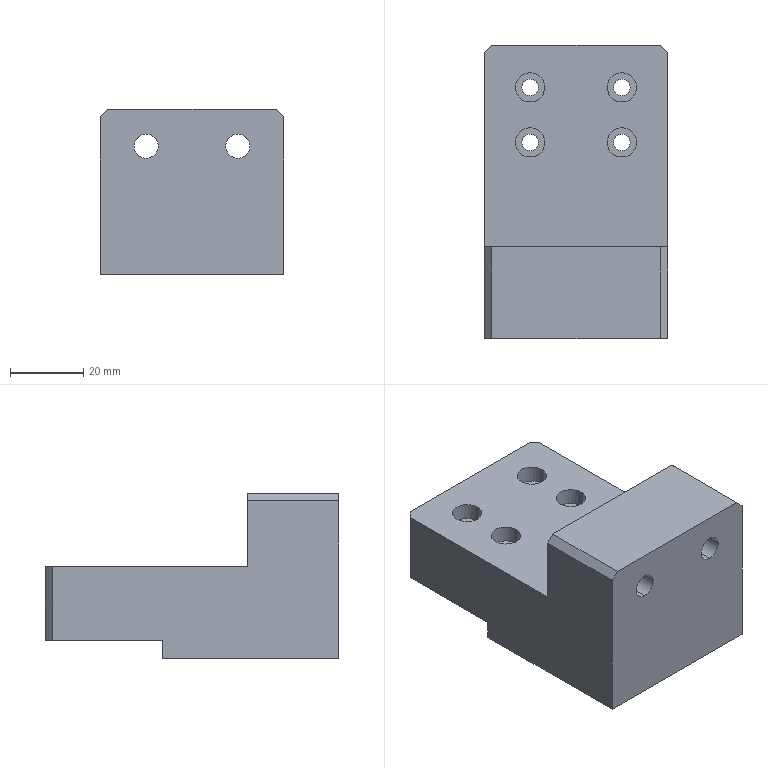Part | STEP file | FBDS-CS-011 | 1 solid | 44 faces | box 50 x 80 x 45 mm | volume 112378 mm3 | cylinder 24 | plane 20 | commonest cylinder face diameters 4.5 x8 8 x8 6.6 x4 11 x4
STEP:
#1=CARTESIAN_POINT('',(-12.5,-21.8,14.5));
#2=VERTEX_POINT('',#1);
#3=CARTESIAN_POINT('',(-12.5,-21.8,25.5));
#4=VERTEX_POINT('',#3);
#5=CARTESIAN_POINT('',(-12.5,-21.8,20.));
#6=DIRECTION('',(0.,1.,0.));
#7=DIRECTION('',(0.,0.,1.));
#8=AXIS2_PLACEMENT_3D('',#5,#6,#7);
#9=CIRCLE('',#8,5.5);
#10=EDGE_CURVE('',#2,#4,#9,.T.);
#11=ORIENTED_EDGE('',*,*,#10,.F.);
#12=CARTESIAN_POINT('',(-12.5,-15.,14.5));
#13=VERTEX_POINT('',#12);
#14=CARTESIAN_POINT('',(-12.5,-15.,14.5));
#15=DIRECTION('',(0.,1.,0.));
#16=VECTOR('',#15,1000.);
#17=LINE('',#14,#16);
#18=EDGE_CURVE('',#2,#13,#17,.T.);
#19=ORIENTED_EDGE('',*,*,#18,.T.);
#20=CARTESIAN_POINT('',(-12.5,-15.,25.5));
#21=VERTEX_POINT('',#20);
#22=CARTESIAN_POINT('',(-12.5,-15.,20.));
#23=DIRECTION('',(0.,1.,0.));
#24=DIRECTION('',(0.,0.,1.));
#25=AXIS2_PLACEMENT_3D('',#22,#23,#24);
#26=CIRCLE('',#25,5.5);
#27=EDGE_CURVE('',#13,#21,#26,.T.);
#28=ORIENTED_EDGE('',*,*,#27,.T.);
#29=CARTESIAN_POINT('',(-12.5,-15.,25.5));
#30=DIRECTION('',(0.,1.,0.));
#31=VECTOR('',#30,1000.);
#32=LINE('',#29,#31);
#33=EDGE_CURVE('',#4,#21,#32,.T.);
#34=ORIENTED_EDGE('',*,*,#33,.F.);
#35=EDGE_LOOP('',(#11,#19,#28,#34));
#36=FACE_OUTER_BOUND('',#35,.T.);
#37=CARTESIAN_POINT('',(-12.5,-15.,20.));
#38=DIRECTION('',(0.,1.,0.));
#39=DIRECTION('',(0.,0.,1.));
#40=AXIS2_PLACEMENT_3D('',#37,#38,#39);
#41=CYLINDRICAL_SURFACE('',#40,5.5);
#42=ADVANCED_FACE('',(#36),#41,.F.);
#43=CARTESIAN_POINT('',(-12.5,-40.,16.7));
#44=VERTEX_POINT('',#43);
#45=CARTESIAN_POINT('',(-12.5,-40.,23.3));
#46=VERTEX_POINT('',#45);
#47=CARTESIAN_POINT('',(-12.5,-40.,20.));
#48=DIRECTION('',(0.,1.,0.));
#49=DIRECTION('',(0.,0.,1.));
#50=AXIS2_PLACEMENT_3D('',#47,#48,#49);
#51=CIRCLE('',#50,3.3);
#52=EDGE_CURVE('',#44,#46,#51,.T.);
#53=ORIENTED_EDGE('',*,*,#52,.F.);
#54=CARTESIAN_POINT('',(-12.5,-21.8,16.7));
#55=VERTEX_POINT('',#54);
#56=CARTESIAN_POINT('',(-12.5,-15.,16.7));
#57=DIRECTION('',(0.,1.,0.));
#58=VECTOR('',#57,1000.);
#59=LINE('',#56,#58);
#60=EDGE_CURVE('',#44,#55,#59,.T.);
#61=ORIENTED_EDGE('',*,*,#60,.T.);
#62=CARTESIAN_POINT('',(-12.5,-21.8,23.3));
#63=VERTEX_POINT('',#62);
#64=CARTESIAN_POINT('',(-12.5,-21.8,20.));
#65=DIRECTION('',(0.,1.,0.));
#66=DIRECTION('',(0.,0.,1.));
#67=AXIS2_PLACEMENT_3D('',#64,#65,#66);
#68=CIRCLE('',#67,3.3);
#69=EDGE_CURVE('',#55,#63,#68,.T.);
#70=ORIENTED_EDGE('',*,*,#69,.T.);
#71=CARTESIAN_POINT('',(-12.5,-15.,23.3));
#72=DIRECTION('',(0.,1.,0.));
#73=VECTOR('',#72,1000.);
#74=LINE('',#71,#73);
#75=EDGE_CURVE('',#46,#63,#74,.T.);
#76=ORIENTED_EDGE('',*,*,#75,.F.);
#77=EDGE_LOOP('',(#53,#61,#70,#76));
#78=FACE_OUTER_BOUND('',#77,.T.);
#79=CARTESIAN_POINT('',(-12.5,-15.,20.));
#80=DIRECTION('',(0.,1.,0.));
#81=DIRECTION('',(0.,0.,1.));
#82=AXIS2_PLACEMENT_3D('',#79,#80,#81);
#83=CYLINDRICAL_SURFACE('',#82,3.3);
#84=ADVANCED_FACE('',(#78),#83,.F.);
#85=CARTESIAN_POINT('',(12.5,-21.8,14.5));
#86=VERTEX_POINT('',#85);
#87=CARTESIAN_POINT('',(12.5,-21.8,25.5));
#88=VERTEX_POINT('',#87);
#89=CARTESIAN_POINT('',(12.5,-21.8,20.));
#90=DIRECTION('',(0.,1.,0.));
#91=DIRECTION('',(0.,0.,1.));
#92=AXIS2_PLACEMENT_3D('',#89,#90,#91);
#93=CIRCLE('',#92,5.5);
#94=EDGE_CURVE('',#86,#88,#93,.T.);
#95=ORIENTED_EDGE('',*,*,#94,.F.);
#96=CARTESIAN_POINT('',(12.5,-15.,14.5));
#97=VERTEX_POINT('',#96);
#98=CARTESIAN_POINT('',(12.5,-15.,14.5));
#99=DIRECTION('',(0.,1.,0.));
#100=VECTOR('',#99,1000.);
#101=LINE('',#98,#100);
#102=EDGE_CURVE('',#86,#97,#101,.T.);
#103=ORIENTED_EDGE('',*,*,#102,.T.);
#104=CARTESIAN_POINT('',(12.5,-15.,25.5));
#105=VERTEX_POINT('',#104);
#106=CARTESIAN_POINT('',(12.5,-15.,20.));
#107=DIRECTION('',(0.,1.,0.));
#108=DIRECTION('',(0.,0.,1.));
#109=AXIS2_PLACEMENT_3D('',#106,#107,#108);
#110=CIRCLE('',#109,5.5);
#111=EDGE_CURVE('',#97,#105,#110,.T.);
#112=ORIENTED_EDGE('',*,*,#111,.T.);
#113=CARTESIAN_POINT('',(12.5,-15.,25.5));
#114=DIRECTION('',(0.,1.,0.));
#115=VECTOR('',#114,1000.);
#116=LINE('',#113,#115);
#117=EDGE_CURVE('',#88,#105,#116,.T.);
#118=ORIENTED_EDGE('',*,*,#117,.F.);
#119=EDGE_LOOP('',(#95,#103,#112,#118));
#120=FACE_OUTER_BOUND('',#119,.T.);
#121=CARTESIAN_POINT('',(12.5,-15.,20.));
#122=DIRECTION('',(0.,1.,0.));
#123=DIRECTION('',(0.,0.,1.));
#124=AXIS2_PLACEMENT_3D('',#121,#122,#123);
#125=CYLINDRICAL_SURFACE('',#124,5.5);
#126=ADVANCED_FACE('',(#120),#125,.F.);
#127=CARTESIAN_POINT('',(12.5,-40.,16.7));
#128=VERTEX_POINT('',#127);
#129=CARTESIAN_POINT('',(12.5,-40.,23.3));
#130=VERTEX_POINT('',#129);
#131=CARTESIAN_POINT('',(12.5,-40.,20.));
#132=DIRECTION('',(0.,1.,0.));
#133=DIRECTION('',(0.,0.,1.));
#134=AXIS2_PLACEMENT_3D('',#131,#132,#133);
#135=CIRCLE('',#134,3.3);
#136=EDGE_CURVE('',#128,#130,#135,.T.);
#137=ORIENTED_EDGE('',*,*,#136,.F.);
#138=CARTESIAN_POINT('',(12.5,-21.8,16.7));
#139=VERTEX_POINT('',#138);
#140=CARTESIAN_POINT('',(12.5,-15.,16.7));
#141=DIRECTION('',(0.,1.,0.));
#142=VECTOR('',#141,1000.);
#143=LINE('',#140,#142);
#144=EDGE_CURVE('',#128,#139,#143,.T.);
#145=ORIENTED_EDGE('',*,*,#144,.T.);
#146=CARTESIAN_POINT('',(12.5,-21.8,23.3));
#147=VERTEX_POINT('',#146);
#148=CARTESIAN_POINT('',(12.5,-21.8,20.));
#149=DIRECTION('',(0.,1.,0.));
#150=DIRECTION('',(0.,0.,1.));
#151=AXIS2_PLACEMENT_3D('',#148,#149,#150);
#152=CIRCLE('',#151,3.3);
#153=EDGE_CURVE('',#139,#147,#152,.T.);
#154=ORIENTED_EDGE('',*,*,#153,.T.);
#155=CARTESIAN_POINT('',(12.5,-15.,23.3));
#156=DIRECTION('',(0.,1.,0.));
#157=VECTOR('',#156,1000.);
#158=LINE('',#155,#157);
#159=EDGE_CURVE('',#130,#147,#158,.T.);
#160=ORIENTED_EDGE('',*,*,#159,.F.);
#161=EDGE_LOOP('',(#137,#145,#154,#160));
#162=FACE_OUTER_BOUND('',#161,.T.);
#163=CARTESIAN_POINT('',(12.5,-15.,20.));
#164=DIRECTION('',(0.,1.,0.));
#165=DIRECTION('',(0.,0.,1.));
#166=AXIS2_PLACEMENT_3D('',#163,#164,#165);
#167=CYLINDRICAL_SURFACE('',#166,3.3);
#168=ADVANCED_FACE('',(#162),#167,.F.);
#169=CARTESIAN_POINT('',(-16.5,28.5,5.4));
#170=VERTEX_POINT('',#169);
#171=CARTESIAN_POINT('',(-8.5,28.5,5.4));
#172=VERTEX_POINT('',#171);
#173=CARTESIAN_POINT('',(-12.5,28.5,5.4));
#174=DIRECTION('',(0.,0.,1.));
#175=DIRECTION('',(1.,0.,0.));
#176=AXIS2_PLACEMENT_3D('',#173,#174,#175);
#177=CIRCLE('',#176,4.);
#178=EDGE_CURVE('',#170,#172,#177,.T.);
#179=ORIENTED_EDGE('',*,*,#178,.F.);
#180=CARTESIAN_POINT('',(-16.5,28.5,10.));
#181=VERTEX_POINT('',#180);
#182=CARTESIAN_POINT('',(-16.5,28.5,10.));
#183=DIRECTION('',(0.,0.,1.));
#184=VECTOR('',#183,1000.);
#185=LINE('',#182,#184);
#186=EDGE_CURVE('',#170,#181,#185,.T.);
#187=ORIENTED_EDGE('',*,*,#186,.T.);
#188=CARTESIAN_POINT('',(-8.5,28.5,10.));
#189=VERTEX_POINT('',#188);
#190=CARTESIAN_POINT('',(-12.5,28.5,10.));
#191=DIRECTION('',(0.,0.,1.));
#192=DIRECTION('',(1.,0.,0.));
#193=AXIS2_PLACEMENT_3D('',#190,#191,#192);
#194=CIRCLE('',#193,4.);
#195=EDGE_CURVE('',#181,#189,#194,.T.);
#196=ORIENTED_EDGE('',*,*,#195,.T.);
#197=CARTESIAN_POINT('',(-8.5,28.5,10.));
#198=DIRECTION('',(0.,0.,1.));
#199=VECTOR('',#198,1000.);
#200=LINE('',#197,#199);
#201=EDGE_CURVE('',#172,#189,#200,.T.);
#202=ORIENTED_EDGE('',*,*,#201,.F.);
#203=EDGE_LOOP('',(#179,#187,#196,#202));
#204=FACE_OUTER_BOUND('',#203,.T.);
#205=CARTESIAN_POINT('',(-12.5,28.5,10.));
#206=DIRECTION('',(0.,0.,1.));
#207=DIRECTION('',(1.,0.,0.));
#208=AXIS2_PLACEMENT_3D('',#205,#206,#207);
#209=CYLINDRICAL_SURFACE('',#208,4.);
#210=ADVANCED_FACE('',(#204),#209,.F.);
#211=CARTESIAN_POINT('',(-14.75,28.5,-10.));
#212=VERTEX_POINT('',#211);
#213=CARTESIAN_POINT('',(-10.25,28.5,-10.));
#214=VERTEX_POINT('',#213);
#215=CARTESIAN_POINT('',(-12.5,28.5,-10.));
#216=DIRECTION('',(0.,0.,1.));
#217=DIRECTION('',(1.,0.,0.));
#218=AXIS2_PLACEMENT_3D('',#215,#216,#217);
#219=CIRCLE('',#218,2.25);
#220=EDGE_CURVE('',#212,#214,#219,.T.);
#221=ORIENTED_EDGE('',*,*,#220,.F.);
#222=CARTESIAN_POINT('',(-14.75,28.5,5.4));
#223=VERTEX_POINT('',#222);
#224=CARTESIAN_POINT('',(-14.75,28.5,10.));
#225=DIRECTION('',(0.,0.,1.));
#226=VECTOR('',#225,1000.);
#227=LINE('',#224,#226);
#228=EDGE_CURVE('',#212,#223,#227,.T.);
#229=ORIENTED_EDGE('',*,*,#228,.T.);
#230=CARTESIAN_POINT('',(-10.25,28.5,5.4));
#231=VERTEX_POINT('',#230);
#232=CARTESIAN_POINT('',(-12.5,28.5,5.4));
#233=DIRECTION('',(0.,0.,1.));
#234=DIRECTION('',(1.,0.,0.));
#235=AXIS2_PLACEMENT_3D('',#232,#233,#234);
#236=CIRCLE('',#235,2.25);
#237=EDGE_CURVE('',#223,#231,#236,.T.);
#238=ORIENTED_EDGE('',*,*,#237,.T.);
#239=CARTESIAN_POINT('',(-10.25,28.5,10.));
#240=DIRECTION('',(0.,0.,1.));
#241=VECTOR('',#240,1000.);
#242=LINE('',#239,#241);
#243=EDGE_CURVE('',#214,#231,#242,.T.);
#244=ORIENTED_EDGE('',*,*,#243,.F.);
#245=EDGE_LOOP('',(#221,#229,#238,#244));
#246=FACE_OUTER_BOUND('',#245,.T.);
#247=CARTESIAN_POINT('',(-12.5,28.5,10.));
#248=DIRECTION('',(0.,0.,1.));
#249=DIRECTION('',(1.,0.,0.));
#250=AXIS2_PLACEMENT_3D('',#247,#248,#249);
#251=CYLINDRICAL_SURFACE('',#250,2.25);
#252=ADVANCED_FACE('',(#246),#251,.F.);
#253=CARTESIAN_POINT('',(8.5,28.5,5.4));
#254=VERTEX_POINT('',#253);
#255=CARTESIAN_POINT('',(16.5,28.5,5.4));
#256=VERTEX_POINT('',#255);
#257=CARTESIAN_POINT('',(12.5,28.5,5.4));
#258=DIRECTION('',(0.,0.,1.));
#259=DIRECTION('',(1.,0.,0.));
#260=AXIS2_PLACEMENT_3D('',#257,#258,#259);
#261=CIRCLE('',#260,4.);
#262=EDGE_CURVE('',#254,#256,#261,.T.);
#263=ORIENTED_EDGE('',*,*,#262,.F.);
#264=CARTESIAN_POINT('',(8.5,28.5,10.));
#265=VERTEX_POINT('',#264);
#266=CARTESIAN_POINT('',(8.5,28.5,10.));
#267=DIRECTION('',(0.,0.,1.));
#268=VECTOR('',#267,1000.);
#269=LINE('',#266,#268);
#270=EDGE_CURVE('',#254,#265,#269,.T.);
#271=ORIENTED_EDGE('',*,*,#270,.T.);
#272=CARTESIAN_POINT('',(16.5,28.5,10.));
#273=VERTEX_POINT('',#272);
#274=CARTESIAN_POINT('',(12.5,28.5,10.));
#275=DIRECTION('',(0.,0.,1.));
#276=DIRECTION('',(1.,0.,0.));
#277=AXIS2_PLACEMENT_3D('',#274,#275,#276);
#278=CIRCLE('',#277,4.);
#279=EDGE_CURVE('',#265,#273,#278,.T.);
#280=ORIENTED_EDGE('',*,*,#279,.T.);
#281=CARTESIAN_POINT('',(16.5,28.5,10.));
#282=DIRECTION('',(0.,0.,1.));
#283=VECTOR('',#282,1000.);
#284=LINE('',#281,#283);
#285=EDGE_CURVE('',#256,#273,#284,.T.);
#286=ORIENTED_EDGE('',*,*,#285,.F.);
#287=EDGE_LOOP('',(#263,#271,#280,#286));
#288=FACE_OUTER_BOUND('',#287,.T.);
#289=CARTESIAN_POINT('',(12.5,28.5,10.));
#290=DIRECTION('',(0.,0.,1.));
#291=DIRECTION('',(1.,0.,0.));
#292=AXIS2_PLACEMENT_3D('',#289,#290,#291);
#293=CYLINDRICAL_SURFACE('',#292,4.);
#294=ADVANCED_FACE('',(#288),#293,.F.);
#295=CARTESIAN_POINT('',(10.25,28.5,-10.));
#296=VERTEX_POINT('',#295);
#297=CARTESIAN_POINT('',(14.75,28.5,-10.));
#298=VERTEX_POINT('',#297);
#299=CARTESIAN_POINT('',(12.5,28.5,-10.));
#300=DIRECTION('',(0.,0.,1.));
#301=DIRECTION('',(1.,0.,0.));
#302=AXIS2_PLACEMENT_3D('',#299,#300,#301);
#303=CIRCLE('',#302,2.25);
#304=EDGE_CURVE('',#296,#298,#303,.T.);
#305=ORIENTED_EDGE('',*,*,#304,.F.);
#306=CARTESIAN_POINT('',(10.25,28.5,5.4));
#307=VERTEX_POINT('',#306);
#308=CARTESIAN_POINT('',(10.25,28.5,10.));
#309=DIRECTION('',(0.,0.,1.));
#310=VECTOR('',#309,1000.);
#311=LINE('',#308,#310);
#312=EDGE_CURVE('',#296,#307,#311,.T.);
#313=ORIENTED_EDGE('',*,*,#312,.T.);
#314=CARTESIAN_POINT('',(14.75,28.5,5.4));
#315=VERTEX_POINT('',#314);
#316=CARTESIAN_POINT('',(12.5,28.5,5.4));
#317=DIRECTION('',(0.,0.,1.));
#318=DIRECTION('',(1.,0.,0.));
#319=AXIS2_PLACEMENT_3D('',#316,#317,#318);
#320=CIRCLE('',#319,2.25);
#321=EDGE_CURVE('',#307,#315,#320,.T.);
#322=ORIENTED_EDGE('',*,*,#321,.T.);
#323=CARTESIAN_POINT('',(14.75,28.5,10.));
#324=DIRECTION('',(0.,0.,1.));
#325=VECTOR('',#324,1000.);
#326=LINE('',#323,#325);
#327=EDGE_CURVE('',#298,#315,#326,.T.);
#328=ORIENTED_EDGE('',*,*,#327,.F.);
#329=EDGE_LOOP('',(#305,#313,#322,#328));
#330=FACE_OUTER_BOUND('',#329,.T.);
#331=CARTESIAN_POINT('',(12.5,28.5,10.));
#332=DIRECTION('',(0.,0.,1.));
#333=DIRECTION('',(1.,0.,0.));
#334=AXIS2_PLACEMENT_3D('',#331,#332,#333);
#335=CYLINDRICAL_SURFACE('',#334,2.25);
#336=ADVANCED_FACE('',(#330),#335,.F.);
#337=CARTESIAN_POINT('',(8.5,13.5,5.4));
#338=VERTEX_POINT('',#337);
#339=CARTESIAN_POINT('',(16.5,13.5,5.4));
#340=VERTEX_POINT('',#339);
#341=CARTESIAN_POINT('',(12.5,13.5,5.4));
#342=DIRECTION('',(0.,0.,1.));
#343=DIRECTION('',(1.,0.,0.));
#344=AXIS2_PLACEMENT_3D('',#341,#342,#343);
#345=CIRCLE('',#344,4.);
#346=EDGE_CURVE('',#338,#340,#345,.T.);
#347=ORIENTED_EDGE('',*,*,#346,.F.);
#348=CARTESIAN_POINT('',(8.5,13.5,10.));
#349=VERTEX_POINT('',#348);
#350=CARTESIAN_POINT('',(8.5,13.5,10.));
#351=DIRECTION('',(0.,0.,1.));
#352=VECTOR('',#351,1000.);
#353=LINE('',#350,#352);
#354=EDGE_CURVE('',#338,#349,#353,.T.);
#355=ORIENTED_EDGE('',*,*,#354,.T.);
#356=CARTESIAN_POINT('',(16.5,13.5,10.));
#357=VERTEX_POINT('',#356);
#358=CARTESIAN_POINT('',(12.5,13.5,10.));
#359=DIRECTION('',(0.,0.,1.));
#360=DIRECTION('',(1.,0.,0.));
#361=AXIS2_PLACEMENT_3D('',#358,#359,#360);
#362=CIRCLE('',#361,4.);
#363=EDGE_CURVE('',#349,#357,#362,.T.);
#364=ORIENTED_EDGE('',*,*,#363,.T.);
#365=CARTESIAN_POINT('',(16.5,13.5,10.));
#366=DIRECTION('',(0.,0.,1.));
#367=VECTOR('',#366,1000.);
#368=LINE('',#365,#367);
#369=EDGE_CURVE('',#340,#357,#368,.T.);
#370=ORIENTED_EDGE('',*,*,#369,.F.);
#371=EDGE_LOOP('',(#347,#355,#364,#370));
#372=FACE_OUTER_BOUND('',#371,.T.);
#373=CARTESIAN_POINT('',(12.5,13.5,10.));
#374=DIRECTION('',(0.,0.,1.));
#375=DIRECTION('',(1.,0.,0.));
#376=AXIS2_PLACEMENT_3D('',#373,#374,#375);
#377=CYLINDRICAL_SURFACE('',#376,4.);
#378=ADVANCED_FACE('',(#372),#377,.F.);
#379=CARTESIAN_POINT('',(10.25,13.5,-10.));
#380=VERTEX_POINT('',#379);
#381=CARTESIAN_POINT('',(14.75,13.5,-10.));
#382=VERTEX_POINT('',#381);
#383=CARTESIAN_POINT('',(12.5,13.5,-10.));
#384=DIRECTION('',(0.,0.,1.));
#385=DIRECTION('',(1.,0.,0.));
#386=AXIS2_PLACEMENT_3D('',#383,#384,#385);
#387=CIRCLE('',#386,2.25);
#388=EDGE_CURVE('',#380,#382,#387,.T.);
#389=ORIENTED_EDGE('',*,*,#388,.F.);
#390=CARTESIAN_POINT('',(10.25,13.5,5.4));
#391=VERTEX_POINT('',#390);
#392=CARTESIAN_POINT('',(10.25,13.5,10.));
#393=DIRECTION('',(0.,0.,1.));
#394=VECTOR('',#393,1000.);
#395=LINE('',#392,#394);
#396=EDGE_CURVE('',#380,#391,#395,.T.);
#397=ORIENTED_EDGE('',*,*,#396,.T.);
#398=CARTESIAN_POINT('',(14.75,13.5,5.4));
#399=VERTEX_POINT('',#398);
#400=CARTESIAN_POINT('',(12.5,13.5,5.4));
#401=DIRECTION('',(0.,0.,1.));
#402=DIRECTION('',(1.,0.,0.));
#403=AXIS2_PLACEMENT_3D('',#400,#401,#402);
#404=CIRCLE('',#403,2.25);
#405=EDGE_CURVE('',#391,#399,#404,.T.);
#406=ORIENTED_EDGE('',*,*,#405,.T.);
#407=CARTESIAN_POINT('',(14.75,13.5,10.));
#408=DIRECTION('',(0.,0.,1.));
#409=VECTOR('',#408,1000.);
#410=LINE('',#407,#409);
#411=EDGE_CURVE('',#382,#399,#410,.T.);
#412=ORIENTED_EDGE('',*,*,#411,.F.);
#413=EDGE_LOOP('',(#389,#397,#406,#412));
#414=FACE_OUTER_BOUND('',#413,.T.);
#415=CARTESIAN_POINT('',(12.5,13.5,10.));
#416=DIRECTION('',(0.,0.,1.));
#417=DIRECTION('',(1.,0.,0.));
#418=AXIS2_PLACEMENT_3D('',#415,#416,#417);
#419=CYLINDRICAL_SURFACE('',#418,2.25);
#420=ADVANCED_FACE('',(#414),#419,.F.);
#421=CARTESIAN_POINT('',(-16.5,13.5,5.4));
#422=VERTEX_POINT('',#421);
#423=CARTESIAN_POINT('',(-8.5,13.5,5.4));
#424=VERTEX_POINT('',#423);
#425=CARTESIAN_POINT('',(-12.5,13.5,5.4));
#426=DIRECTION('',(0.,0.,1.));
#427=DIRECTION('',(1.,0.,0.));
#428=AXIS2_PLACEMENT_3D('',#425,#426,#427);
#429=CIRCLE('',#428,4.);
#430=EDGE_CURVE('',#422,#424,#429,.T.);
#431=ORIENTED_EDGE('',*,*,#430,.F.);
#432=CARTESIAN_POINT('',(-16.5,13.5,10.));
#433=VERTEX_POINT('',#432);
#434=CARTESIAN_POINT('',(-16.5,13.5,10.));
#435=DIRECTION('',(0.,0.,1.));
#436=VECTOR('',#435,1000.);
#437=LINE('',#434,#436);
#438=EDGE_CURVE('',#422,#433,#437,.T.);
#439=ORIENTED_EDGE('',*,*,#438,.T.);
#440=CARTESIAN_POINT('',(-8.5,13.5,10.));
#441=VERTEX_POINT('',#440);
#442=CARTESIAN_POINT('',(-12.5,13.5,10.));
#443=DIRECTION('',(0.,0.,1.));
#444=DIRECTION('',(1.,0.,0.));
#445=AXIS2_PLACEMENT_3D('',#442,#443,#444);
#446=CIRCLE('',#445,4.);
#447=EDGE_CURVE('',#433,#441,#446,.T.);
#448=ORIENTED_EDGE('',*,*,#447,.T.);
#449=CARTESIAN_POINT('',(-8.5,13.5,10.));
#450=DIRECTION('',(0.,0.,1.));
#451=VECTOR('',#450,1000.);
#452=LINE('',#449,#451);
#453=EDGE_CURVE('',#424,#441,#452,.T.);
#454=ORIENTED_EDGE('',*,*,#453,.F.);
#455=EDGE_LOOP('',(#431,#439,#448,#454));
#456=FACE_OUTER_BOUND('',#455,.T.);
#457=CARTESIAN_POINT('',(-12.5,13.5,10.));
#458=DIRECTION('',(0.,0.,1.));
#459=DIRECTION('',(1.,0.,0.));
#460=AXIS2_PLACEMENT_3D('',#457,#458,#459);
#461=CYLINDRICAL_SURFACE('',#460,4.);
#462=ADVANCED_FACE('',(#456),#461,.F.);
#463=CARTESIAN_POINT('',(-14.75,13.5,-10.));
#464=VERTEX_POINT('',#463);
#465=CARTESIAN_POINT('',(-10.25,13.5,-10.));
#466=VERTEX_POINT('',#465);
#467=CARTESIAN_POINT('',(-12.5,13.5,-10.));
#468=DIRECTION('',(0.,0.,1.));
#469=DIRECTION('',(1.,0.,0.));
#470=AXIS2_PLACEMENT_3D('',#467,#468,#469);
#471=CIRCLE('',#470,2.25);
#472=EDGE_CURVE('',#464,#466,#471,.T.);
#473=ORIENTED_EDGE('',*,*,#472,.F.);
#474=CARTESIAN_POINT('',(-14.75,13.5,5.4));
#475=VERTEX_POINT('',#474);
#476=CARTESIAN_POINT('',(-14.75,13.5,10.));
#477=DIRECTION('',(0.,0.,1.));
#478=VECTOR('',#477,1000.);
#479=LINE('',#476,#478);
#480=EDGE_CURVE('',#464,#475,#479,.T.);
#481=ORIENTED_EDGE('',*,*,#480,.T.);
#482=CARTESIAN_POINT('',(-10.25,13.5,5.4));
#483=VERTEX_POINT('',#482);
#484=CARTESIAN_POINT('',(-12.5,13.5,5.4));
#485=DIRECTION('',(0.,0.,1.));
#486=DIRECTION('',(1.,0.,0.));
#487=AXIS2_PLACEMENT_3D('',#484,#485,#486);
#488=CIRCLE('',#487,2.25);
#489=EDGE_CURVE('',#475,#483,#488,.T.);
#490=ORIENTED_EDGE('',*,*,#489,.T.);
#491=CARTESIAN_POINT('',(-10.25,13.5,10.));
#492=DIRECTION('',(0.,0.,1.));
#493=VECTOR('',#492,1000.);
#494=LINE('',#491,#493);
#495=EDGE_CURVE('',#466,#483,#494,.T.);
#496=ORIENTED_EDGE('',*,*,#495,.F.);
#497=EDGE_LOOP('',(#473,#481,#490,#496));
#498=FACE_OUTER_BOUND('',#497,.T.);
#499=CARTESIAN_POINT('',(-12.5,13.5,10.));
#500=DIRECTION('',(0.,0.,1.));
#501=DIRECTION('',(1.,0.,0.));
#502=AXIS2_PLACEMENT_3D('',#499,#500,#501);
#503=CYLINDRICAL_SURFACE('',#502,2.25);
#504=ADVANCED_FACE('',(#498),#503,.F.);
#505=CARTESIAN_POINT('',(-12.5,-15.,20.));
#506=DIRECTION('',(0.,1.,0.));
#507=DIRECTION('',(0.,0.,1.));
#508=AXIS2_PLACEMENT_3D('',#505,#506,#507);
#509=CIRCLE('',#508,5.5);
#510=EDGE_CURVE('',#21,#13,#509,.T.);
#511=ORIENTED_EDGE('',*,*,#510,.F.);
#512=ORIENTED_EDGE('',*,*,#27,.F.);
#513=EDGE_LOOP('',(#511,#512));
#514=FACE_BOUND('',#513,.T.);
#515=CARTESIAN_POINT('',(-25.,-15.,28.));
#516=VERTEX_POINT('',#515);
#517=CARTESIAN_POINT('',(-25.,-15.,10.));
#518=VERTEX_POINT('',#517);
#519=CARTESIAN_POINT('',(-25.,-15.,30.));
#520=DIRECTION('',(0.,0.,-1.));
#521=VECTOR('',#520,1000.);
#522=LINE('',#519,#521);
#523=EDGE_CURVE('',#516,#518,#522,.T.);
#524=ORIENTED_EDGE('',*,*,#523,.F.);
#525=CARTESIAN_POINT('',(-23.,-15.,30.));
#526=VERTEX_POINT('',#525);
#527=CARTESIAN_POINT('',(-23.,-15.,30.));
#528=DIRECTION('',(0.7071,0.,0.7071));
#529=VECTOR('',#528,1000.);
#530=LINE('',#527,#529);
#531=EDGE_CURVE('',#516,#526,#530,.T.);
#532=ORIENTED_EDGE('',*,*,#531,.T.);
#533=CARTESIAN_POINT('',(23.,-15.,30.));
#534=VERTEX_POINT('',#533);
#535=CARTESIAN_POINT('',(-25.,-15.,30.));
#536=DIRECTION('',(-1.,0.,0.));
#537=VECTOR('',#536,1000.);
#538=LINE('',#535,#537);
#539=EDGE_CURVE('',#534,#526,#538,.T.);
#540=ORIENTED_EDGE('',*,*,#539,.F.);
#541=CARTESIAN_POINT('',(25.,-15.,28.));
#542=VERTEX_POINT('',#541);
#543=CARTESIAN_POINT('',(23.,-15.,30.));
#544=DIRECTION('',(0.7071,0.,-0.7071));
#545=VECTOR('',#544,1000.);
#546=LINE('',#543,#545);
#547=EDGE_CURVE('',#534,#542,#546,.T.);
#548=ORIENTED_EDGE('',*,*,#547,.T.);
#549=CARTESIAN_POINT('',(25.,-15.,10.));
#550=VERTEX_POINT('',#549);
#551=CARTESIAN_POINT('',(25.,-15.,30.));
#552=DIRECTION('',(0.,0.,-1.));
#553=VECTOR('',#552,1000.);
#554=LINE('',#551,#553);
#555=EDGE_CURVE('',#542,#550,#554,.T.);
#556=ORIENTED_EDGE('',*,*,#555,.T.);
#557=CARTESIAN_POINT('',(-25.,-15.,10.));
#558=DIRECTION('',(-1.,0.,0.));
#559=VECTOR('',#558,1000.);
#560=LINE('',#557,#559);
#561=EDGE_CURVE('',#550,#518,#560,.T.);
#562=ORIENTED_EDGE('',*,*,#561,.T.);
#563=EDGE_LOOP('',(#524,#532,#540,#548,#556,#562));
#564=FACE_OUTER_BOUND('',#563,.T.);
#565=CARTESIAN_POINT('',(12.5,-15.,20.));
#566=DIRECTION('',(0.,1.,0.));
#567=DIRECTION('',(0.,0.,1.));
#568=AXIS2_PLACEMENT_3D('',#565,#566,#567);
#569=CIRCLE('',#568,5.5);
#570=EDGE_CURVE('',#105,#97,#569,.T.);
#571=ORIENTED_EDGE('',*,*,#570,.F.);
#572=ORIENTED_EDGE('',*,*,#111,.F.);
#573=EDGE_LOOP('',(#571,#572));
#574=FACE_BOUND('',#573,.T.);
#575=CARTESIAN_POINT('',(-25.,-15.,30.));
#576=DIRECTION('',(0.,-1.,0.));
#577=DIRECTION('',(0.,0.,-1.));
#578=AXIS2_PLACEMENT_3D('',#575,#576,#577);
#579=PLANE('',#578);
#580=ADVANCED_FACE('',(#514,#564,#574),#579,.F.);
#581=CARTESIAN_POINT('',(-12.5,13.5,-10.));
#582=DIRECTION('',(0.,0.,1.));
#583=DIRECTION('',(1.,0.,0.));
#584=AXIS2_PLACEMENT_3D('',#581,#582,#583);
#585=CIRCLE('',#584,2.25);
#586=EDGE_CURVE('',#466,#464,#585,.T.);
#587=ORIENTED_EDGE('',*,*,#586,.T.);
#588=ORIENTED_EDGE('',*,*,#472,.T.);
#589=EDGE_LOOP('',(#587,#588));
#590=FACE_BOUND('',#589,.T.);
#591=CARTESIAN_POINT('',(12.5,13.5,-10.));
#592=DIRECTION('',(0.,0.,1.));
#593=DIRECTION('',(1.,0.,0.));
#594=AXIS2_PLACEMENT_3D('',#591,#592,#593);
#595=CIRCLE('',#594,2.25);
#596=EDGE_CURVE('',#382,#380,#595,.T.);
#597=ORIENTED_EDGE('',*,*,#596,.T.);
#598=ORIENTED_EDGE('',*,*,#388,.T.);
#599=EDGE_LOOP('',(#597,#598));
#600=FACE_BOUND('',#599,.T.);
#601=CARTESIAN_POINT('',(12.5,28.5,-10.));
#602=DIRECTION('',(0.,0.,1.));
#603=DIRECTION('',(1.,0.,0.));
#604=AXIS2_PLACEMENT_3D('',#601,#602,#603);
#605=CIRCLE('',#604,2.25);
#606=EDGE_CURVE('',#298,#296,#605,.T.);
#607=ORIENTED_EDGE('',*,*,#606,.T.);
#608=ORIENTED_EDGE('',*,*,#304,.T.);
#609=EDGE_LOOP('',(#607,#608));
#610=FACE_BOUND('',#609,.T.);
#611=CARTESIAN_POINT('',(-12.5,28.5,-10.));
#612=DIRECTION('',(0.,0.,1.));
#613=DIRECTION('',(1.,0.,0.));
#614=AXIS2_PLACEMENT_3D('',#611,#612,#613);
#615=CIRCLE('',#614,2.25);
#616=EDGE_CURVE('',#214,#212,#615,.T.);
#617=ORIENTED_EDGE('',*,*,#616,.T.);
#618=ORIENTED_EDGE('',*,*,#220,.T.);
#619=EDGE_LOOP('',(#617,#618));
#620=FACE_BOUND('',#619,.T.);
#621=CARTESIAN_POINT('',(23.,40.,-10.));
#622=VERTEX_POINT('',#621);
#623=CARTESIAN_POINT('',(-23.,40.,-10.));
#624=VERTEX_POINT('',#623);
#625=CARTESIAN_POINT('',(-25.,40.,-10.));
#626=DIRECTION('',(-1.,0.,0.));
#627=VECTOR('',#626,1000.);
#628=LINE('',#625,#627);
#629=EDGE_CURVE('',#622,#624,#628,.T.);
#630=ORIENTED_EDGE('',*,*,#629,.F.);
#631=CARTESIAN_POINT('',(25.,38.,-10.));
#632=VERTEX_POINT('',#631);
#633=CARTESIAN_POINT('',(23.,40.,-10.));
#634=DIRECTION('',(0.7071,-0.7071,0.));
#635=VECTOR('',#634,1000.);
#636=LINE('',#633,#635);
#637=EDGE_CURVE('',#622,#632,#636,.T.);
#638=ORIENTED_EDGE('',*,*,#637,.T.);
#639=CARTESIAN_POINT('',(25.,8.,-10.));
#640=VERTEX_POINT('',#639);
#641=CARTESIAN_POINT('',(25.,40.,-10.));
#642=DIRECTION('',(0.,1.,0.));
#643=VECTOR('',#642,1000.);
#644=LINE('',#641,#643);
#645=EDGE_CURVE('',#640,#632,#644,.T.);
#646=ORIENTED_EDGE('',*,*,#645,.F.);
#647=CARTESIAN_POINT('',(-25.,8.,-10.));
#648=VERTEX_POINT('',#647);
#649=CARTESIAN_POINT('',(25.,8.,-10.));
#650=DIRECTION('',(1.,0.,0.));
#651=VECTOR('',#650,1000.);
#652=LINE('',#649,#651);
#653=EDGE_CURVE('',#648,#640,#652,.T.);
#654=ORIENTED_EDGE('',*,*,#653,.F.);
#655=CARTESIAN_POINT('',(-25.,38.,-10.));
#656=VERTEX_POINT('',#655);
#657=CARTESIAN_POINT('',(-25.,40.,-10.));
#658=DIRECTION('',(0.,-1.,0.));
#659=VECTOR('',#658,1000.);
#660=LINE('',#657,#659);
#661=EDGE_CURVE('',#656,#648,#660,.T.);
#662=ORIENTED_EDGE('',*,*,#661,.F.);
#663=CARTESIAN_POINT('',(-25.,38.,-10.));
#664=DIRECTION('',(0.7071,0.7071,0.));
#665=VECTOR('',#664,1000.);
#666=LINE('',#663,#665);
#667=EDGE_CURVE('',#656,#624,#666,.T.);
#668=ORIENTED_EDGE('',*,*,#667,.T.);
#669=EDGE_LOOP('',(#630,#638,#646,#654,#662,#668));
#670=FACE_OUTER_BOUND('',#669,.T.);
#671=CARTESIAN_POINT('',(0.,0.,-10.));
#672=DIRECTION('',(0.,0.,1.));
#673=DIRECTION('',(1.,0.,0.));
#674=AXIS2_PLACEMENT_3D('',#671,#672,#673);
#675=PLANE('',#674);
#676=ADVANCED_FACE('',(#590,#600,#610,#620,#670),#675,.F.);
#677=CARTESIAN_POINT('',(-25.,-40.,28.));
#678=VERTEX_POINT('',#677);
#679=CARTESIAN_POINT('',(-25.,-40.,-15.));
#680=VERTEX_POINT('',#679);
#681=CARTESIAN_POINT('',(-25.,-40.,10.));
#682=DIRECTION('',(0.,0.,-1.));
#683=VECTOR('',#682,1000.);
#684=LINE('',#681,#683);
#685=EDGE_CURVE('',#678,#680,#684,.T.);
#686=ORIENTED_EDGE('',*,*,#685,.F.);
#687=CARTESIAN_POINT('',(-25.,-15.,28.));
#688=DIRECTION('',(0.,1.,0.));
#689=VECTOR('',#688,1000.);
#690=LINE('',#687,#689);
#691=EDGE_CURVE('',#678,#516,#690,.T.);
#692=ORIENTED_EDGE('',*,*,#691,.T.);
#693=ORIENTED_EDGE('',*,*,#523,.T.);
#694=CARTESIAN_POINT('',(-25.,38.,10.));
#695=VERTEX_POINT('',#694);
#696=CARTESIAN_POINT('',(-25.,40.,10.));
#697=DIRECTION('',(0.,-1.,0.));
#698=VECTOR('',#697,1000.);
#699=LINE('',#696,#698);
#700=EDGE_CURVE('',#695,#518,#699,.T.);
#701=ORIENTED_EDGE('',*,*,#700,.F.);
#702=CARTESIAN_POINT('',(-25.,38.,10.));
#703=DIRECTION('',(0.,0.,-1.));
#704=VECTOR('',#703,1000.);
#705=LINE('',#702,#704);
#706=EDGE_CURVE('',#695,#656,#705,.T.);
#707=ORIENTED_EDGE('',*,*,#706,.T.);
#708=ORIENTED_EDGE('',*,*,#661,.T.);
#709=CARTESIAN_POINT('',(-25.,8.,-15.));
#710=VERTEX_POINT('',#709);
#711=CARTESIAN_POINT('',(-25.,8.,-15.));
#712=DIRECTION('',(0.,0.,1.));
#713=VECTOR('',#712,1000.);
#714=LINE('',#711,#713);
#715=EDGE_CURVE('',#710,#648,#714,.T.);
#716=ORIENTED_EDGE('',*,*,#715,.F.);
#717=CARTESIAN_POINT('',(-25.,-40.,-15.));
#718=DIRECTION('',(0.,1.,0.));
#719=VECTOR('',#718,1000.);
#720=LINE('',#717,#719);
#721=EDGE_CURVE('',#680,#710,#720,.T.);
#722=ORIENTED_EDGE('',*,*,#721,.F.);
#723=EDGE_LOOP('',(#686,#692,#693,#701,#707,#708,#716,#722));
#724=FACE_OUTER_BOUND('',#723,.T.);
#725=CARTESIAN_POINT('',(-25.,40.,10.));
#726=DIRECTION('',(1.,0.,0.));
#727=DIRECTION('',(0.,1.,0.));
#728=AXIS2_PLACEMENT_3D('',#725,#726,#727);
#729=PLANE('',#728);
#730=ADVANCED_FACE('',(#724),#729,.F.);
#731=CARTESIAN_POINT('',(-12.5,-40.,20.));
#732=DIRECTION('',(0.,1.,0.));
#733=DIRECTION('',(0.,0.,1.));
#734=AXIS2_PLACEMENT_3D('',#731,#732,#733);
#735=CIRCLE('',#734,3.3);
#736=EDGE_CURVE('',#46,#44,#735,.T.);
#737=ORIENTED_EDGE('',*,*,#736,.T.);
#738=ORIENTED_EDGE('',*,*,#52,.T.);
#739=EDGE_LOOP('',(#737,#738));
#740=FACE_BOUND('',#739,.T.);
#741=CARTESIAN_POINT('',(12.5,-40.,20.));
#742=DIRECTION('',(0.,1.,0.));
#743=DIRECTION('',(0.,0.,1.));
#744=AXIS2_PLACEMENT_3D('',#741,#742,#743);
#745=CIRCLE('',#744,3.3);
#746=EDGE_CURVE('',#130,#128,#745,.T.);
#747=ORIENTED_EDGE('',*,*,#746,.T.);
#748=ORIENTED_EDGE('',*,*,#136,.T.);
#749=EDGE_LOOP('',(#747,#748));
#750=FACE_BOUND('',#749,.T.);
#751=CARTESIAN_POINT('',(-23.,-40.,30.));
#752=VERTEX_POINT('',#751);
#753=CARTESIAN_POINT('',(23.,-40.,30.));
#754=VERTEX_POINT('',#753);
#755=CARTESIAN_POINT('',(-25.,-40.,30.));
#756=DIRECTION('',(1.,0.,0.));
#757=VECTOR('',#756,1000.);
#758=LINE('',#755,#757);
#759=EDGE_CURVE('',#752,#754,#758,.T.);
#760=ORIENTED_EDGE('',*,*,#759,.F.);
#761=CARTESIAN_POINT('',(-23.,-40.,30.));
#762=DIRECTION('',(-0.7071,0.,-0.7071));
#763=VECTOR('',#762,1000.);
#764=LINE('',#761,#763);
#765=EDGE_CURVE('',#752,#678,#764,.T.);
#766=ORIENTED_EDGE('',*,*,#765,.T.);
#767=ORIENTED_EDGE('',*,*,#685,.T.);
#768=CARTESIAN_POINT('',(25.,-40.,-15.));
#769=VERTEX_POINT('',#768);
#770=CARTESIAN_POINT('',(25.,-40.,-15.));
#771=DIRECTION('',(-1.,0.,0.));
#772=VECTOR('',#771,1000.);
#773=LINE('',#770,#772);
#774=EDGE_CURVE('',#769,#680,#773,.T.);
#775=ORIENTED_EDGE('',*,*,#774,.F.);
#776=CARTESIAN_POINT('',(25.,-40.,28.));
#777=VERTEX_POINT('',#776);
#778=CARTESIAN_POINT('',(25.,-40.,10.));
#779=DIRECTION('',(0.,0.,-1.));
#780=VECTOR('',#779,1000.);
#781=LINE('',#778,#780);
#782=EDGE_CURVE('',#777,#769,#781,.T.);
#783=ORIENTED_EDGE('',*,*,#782,.F.);
#784=CARTESIAN_POINT('',(23.,-40.,30.));
#785=DIRECTION('',(-0.7071,0.,0.7071));
#786=VECTOR('',#785,1000.);
#787=LINE('',#784,#786);
#788=EDGE_CURVE('',#777,#754,#787,.T.);
#789=ORIENTED_EDGE('',*,*,#788,.T.);
#790=EDGE_LOOP('',(#760,#766,#767,#775,#783,#789));
#791=FACE_OUTER_BOUND('',#790,.T.);
#792=CARTESIAN_POINT('',(-25.,-40.,10.));
#793=DIRECTION('',(0.,1.,0.));
#794=DIRECTION('',(0.,0.,1.));
#795=AXIS2_PLACEMENT_3D('',#792,#793,#794);
#796=PLANE('',#795);
#797=ADVANCED_FACE('',(#740,#750,#791),#796,.F.);
#798=ORIENTED_EDGE('',*,*,#555,.F.);
#799=CARTESIAN_POINT('',(25.,-40.,28.));
#800=DIRECTION('',(0.,-1.,0.));
#801=VECTOR('',#800,1000.);
#802=LINE('',#799,#801);
#803=EDGE_CURVE('',#542,#777,#802,.T.);
#804=ORIENTED_EDGE('',*,*,#803,.T.);
#805=ORIENTED_EDGE('',*,*,#782,.T.);
#806=CARTESIAN_POINT('',(25.,8.,-15.));
#807=VERTEX_POINT('',#806);
#808=CARTESIAN_POINT('',(25.,-40.,-15.));
#809=DIRECTION('',(0.,-1.,0.));
#810=VECTOR('',#809,1000.);
#811=LINE('',#808,#810);
#812=EDGE_CURVE('',#807,#769,#811,.T.);
#813=ORIENTED_EDGE('',*,*,#812,.F.);
#814=CARTESIAN_POINT('',(25.,8.,-15.));
#815=DIRECTION('',(0.,0.,1.));
#816=VECTOR('',#815,1000.);
#817=LINE('',#814,#816);
#818=EDGE_CURVE('',#807,#640,#817,.T.);
#819=ORIENTED_EDGE('',*,*,#818,.T.);
#820=ORIENTED_EDGE('',*,*,#645,.T.);
#821=CARTESIAN_POINT('',(25.,38.,10.));
#822=VERTEX_POINT('',#821);
#823=CARTESIAN_POINT('',(25.,38.,10.));
#824=DIRECTION('',(0.,0.,1.));
#825=VECTOR('',#824,1000.);
#826=LINE('',#823,#825);
#827=EDGE_CURVE('',#632,#822,#826,.T.);
#828=ORIENTED_EDGE('',*,*,#827,.T.);
#829=CARTESIAN_POINT('',(25.,40.,10.));
#830=DIRECTION('',(0.,1.,0.));
#831=VECTOR('',#830,1000.);
#832=LINE('',#829,#831);
#833=EDGE_CURVE('',#550,#822,#832,.T.);
#834=ORIENTED_EDGE('',*,*,#833,.F.);
#835=EDGE_LOOP('',(#798,#804,#805,#813,#819,#820,#828,#834));
#836=FACE_OUTER_BOUND('',#835,.T.);
#837=CARTESIAN_POINT('',(25.,40.,10.));
#838=DIRECTION('',(-1.,0.,0.));
#839=DIRECTION('',(0.,-1.,0.));
#840=AXIS2_PLACEMENT_3D('',#837,#838,#839);
#841=PLANE('',#840);
#842=ADVANCED_FACE('',(#836),#841,.F.);
#843=CARTESIAN_POINT('',(23.,40.,10.));
#844=VERTEX_POINT('',#843);
#845=CARTESIAN_POINT('',(-23.,40.,10.));
#846=VERTEX_POINT('',#845);
#847=CARTESIAN_POINT('',(-25.,40.,10.));
#848=DIRECTION('',(-1.,0.,0.));
#849=VECTOR('',#848,1000.);
#850=LINE('',#847,#849);
#851=EDGE_CURVE('',#844,#846,#850,.T.);
#852=ORIENTED_EDGE('',*,*,#851,.F.);
#853=CARTESIAN_POINT('',(23.,40.,10.));
#854=DIRECTION('',(0.,0.,-1.));
#855=VECTOR('',#854,1000.);
#856=LINE('',#853,#855);
#857=EDGE_CURVE('',#844,#622,#856,.T.);
#858=ORIENTED_EDGE('',*,*,#857,.T.);
#859=ORIENTED_EDGE('',*,*,#629,.T.);
#860=CARTESIAN_POINT('',(-23.,40.,10.));
#861=DIRECTION('',(0.,0.,1.));
#862=VECTOR('',#861,1000.);
#863=LINE('',#860,#862);
#864=EDGE_CURVE('',#624,#846,#863,.T.);
#865=ORIENTED_EDGE('',*,*,#864,.T.);
#866=EDGE_LOOP('',(#852,#858,#859,#865));
#867=FACE_OUTER_BOUND('',#866,.T.);
#868=CARTESIAN_POINT('',(-25.,40.,10.));
#869=DIRECTION('',(0.,-1.,0.));
#870=DIRECTION('',(0.,0.,-1.));
#871=AXIS2_PLACEMENT_3D('',#868,#869,#870);
#872=PLANE('',#871);
#873=ADVANCED_FACE('',(#867),#872,.F.);
#874=ORIENTED_EDGE('',*,*,#833,.T.);
#875=CARTESIAN_POINT('',(31.5,31.5,10.));
#876=DIRECTION('',(-0.7071,0.7071,0.));
#877=VECTOR('',#876,1000.);
#878=LINE('',#875,#877);
#879=EDGE_CURVE('',#822,#844,#878,.T.);
#880=ORIENTED_EDGE('',*,*,#879,.T.);
#881=ORIENTED_EDGE('',*,*,#851,.T.);
#882=CARTESIAN_POINT('',(-31.5,31.5,10.));
#883=DIRECTION('',(-0.7071,-0.7071,0.));
#884=VECTOR('',#883,1000.);
#885=LINE('',#882,#884);
#886=EDGE_CURVE('',#846,#695,#885,.T.);
#887=ORIENTED_EDGE('',*,*,#886,.T.);
#888=ORIENTED_EDGE('',*,*,#700,.T.);
#889=ORIENTED_EDGE('',*,*,#561,.F.);
#890=EDGE_LOOP('',(#874,#880,#881,#887,#888,#889));
#891=FACE_OUTER_BOUND('',#890,.T.);
#892=CARTESIAN_POINT('',(-12.5,28.5,10.));
#893=DIRECTION('',(0.,0.,1.));
#894=DIRECTION('',(1.,0.,0.));
#895=AXIS2_PLACEMENT_3D('',#892,#893,#894);
#896=CIRCLE('',#895,4.);
#897=EDGE_CURVE('',#189,#181,#896,.T.);
#898=ORIENTED_EDGE('',*,*,#897,.F.);
#899=ORIENTED_EDGE('',*,*,#195,.F.);
#900=EDGE_LOOP('',(#898,#899));
#901=FACE_BOUND('',#900,.T.);
#902=CARTESIAN_POINT('',(12.5,28.5,10.));
#903=DIRECTION('',(0.,0.,1.));
#904=DIRECTION('',(1.,0.,0.));
#905=AXIS2_PLACEMENT_3D('',#902,#903,#904);
#906=CIRCLE('',#905,4.);
#907=EDGE_CURVE('',#273,#265,#906,.T.);
#908=ORIENTED_EDGE('',*,*,#907,.F.);
#909=ORIENTED_EDGE('',*,*,#279,.F.);
#910=EDGE_LOOP('',(#908,#909));
#911=FACE_BOUND('',#910,.T.);
#912=CARTESIAN_POINT('',(12.5,13.5,10.));
#913=DIRECTION('',(0.,0.,1.));
#914=DIRECTION('',(1.,0.,0.));
#915=AXIS2_PLACEMENT_3D('',#912,#913,#914);
#916=CIRCLE('',#915,4.);
#917=EDGE_CURVE('',#357,#349,#916,.T.);
#918=ORIENTED_EDGE('',*,*,#917,.F.);
#919=ORIENTED_EDGE('',*,*,#363,.F.);
#920=EDGE_LOOP('',(#918,#919));
#921=FACE_BOUND('',#920,.T.);
#922=CARTESIAN_POINT('',(-12.5,13.5,10.));
#923=DIRECTION('',(0.,0.,1.));
#924=DIRECTION('',(1.,0.,0.));
#925=AXIS2_PLACEMENT_3D('',#922,#923,#924);
#926=CIRCLE('',#925,4.);
#927=EDGE_CURVE('',#441,#433,#926,.T.);
#928=ORIENTED_EDGE('',*,*,#927,.F.);
#929=ORIENTED_EDGE('',*,*,#447,.F.);
#930=EDGE_LOOP('',(#928,#929));
#931=FACE_BOUND('',#930,.T.);
#932=CARTESIAN_POINT('',(0.,0.,10.));
#933=DIRECTION('',(0.,0.,1.));
#934=DIRECTION('',(1.,0.,0.));
#935=AXIS2_PLACEMENT_3D('',#932,#933,#934);
#936=PLANE('',#935);
#937=ADVANCED_FACE('',(#891,#901,#911,#921,#931),#936,.T.);
#938=ORIENTED_EDGE('',*,*,#480,.F.);
#939=ORIENTED_EDGE('',*,*,#586,.F.);
#940=ORIENTED_EDGE('',*,*,#495,.T.);
#941=CARTESIAN_POINT('',(-12.5,13.5,5.4));
#942=DIRECTION('',(0.,0.,1.));
#943=DIRECTION('',(1.,0.,0.));
#944=AXIS2_PLACEMENT_3D('',#941,#942,#943);
#945=CIRCLE('',#944,2.25);
#946=EDGE_CURVE('',#483,#475,#945,.T.);
#947=ORIENTED_EDGE('',*,*,#946,.T.);
#948=EDGE_LOOP('',(#938,#939,#940,#947));
#949=FACE_OUTER_BOUND('',#948,.T.);
#950=CARTESIAN_POINT('',(-12.5,13.5,10.));
#951=DIRECTION('',(0.,0.,1.));
#952=DIRECTION('',(1.,0.,0.));
#953=AXIS2_PLACEMENT_3D('',#950,#951,#952);
#954=CYLINDRICAL_SURFACE('',#953,2.25);
#955=ADVANCED_FACE('',(#949),#954,.F.);
#956=ORIENTED_EDGE('',*,*,#946,.F.);
#957=ORIENTED_EDGE('',*,*,#489,.F.);
#958=EDGE_LOOP('',(#956,#957));
#959=FACE_BOUND('',#958,.T.);
#960=CARTESIAN_POINT('',(-12.5,13.5,5.4));
#961=DIRECTION('',(0.,0.,1.));
#962=DIRECTION('',(1.,0.,0.));
#963=AXIS2_PLACEMENT_3D('',#960,#961,#962);
#964=CIRCLE('',#963,4.);
#965=EDGE_CURVE('',#424,#422,#964,.T.);
#966=ORIENTED_EDGE('',*,*,#965,.T.);
#967=ORIENTED_EDGE('',*,*,#430,.T.);
#968=EDGE_LOOP('',(#966,#967));
#969=FACE_OUTER_BOUND('',#968,.T.);
#970=CARTESIAN_POINT('',(-10.25,13.5,5.4));
#971=DIRECTION('',(0.,0.,-1.));
#972=DIRECTION('',(-1.,0.,0.));
#973=AXIS2_PLACEMENT_3D('',#970,#971,#972);
#974=PLANE('',#973);
#975=ADVANCED_FACE('',(#959,#969),#974,.F.);
#976=ORIENTED_EDGE('',*,*,#438,.F.);
#977=ORIENTED_EDGE('',*,*,#965,.F.);
#978=ORIENTED_EDGE('',*,*,#453,.T.);
#979=ORIENTED_EDGE('',*,*,#927,.T.);
#980=EDGE_LOOP('',(#976,#977,#978,#979));
#981=FACE_OUTER_BOUND('',#980,.T.);
#982=CARTESIAN_POINT('',(-12.5,13.5,10.));
#983=DIRECTION('',(0.,0.,1.));
#984=DIRECTION('',(1.,0.,0.));
#985=AXIS2_PLACEMENT_3D('',#982,#983,#984);
#986=CYLINDRICAL_SURFACE('',#985,4.);
#987=ADVANCED_FACE('',(#981),#986,.F.);
#988=ORIENTED_EDGE('',*,*,#396,.F.);
#989=ORIENTED_EDGE('',*,*,#596,.F.);
#990=ORIENTED_EDGE('',*,*,#411,.T.);
#991=CARTESIAN_POINT('',(12.5,13.5,5.4));
#992=DIRECTION('',(0.,0.,1.));
#993=DIRECTION('',(1.,0.,0.));
#994=AXIS2_PLACEMENT_3D('',#991,#992,#993);
#995=CIRCLE('',#994,2.25);
#996=EDGE_CURVE('',#399,#391,#995,.T.);
#997=ORIENTED_EDGE('',*,*,#996,.T.);
#998=EDGE_LOOP('',(#988,#989,#990,#997));
#999=FACE_OUTER_BOUND('',#998,.T.);
#1000=CARTESIAN_POINT('',(12.5,13.5,10.));
#1001=DIRECTION('',(0.,0.,1.));
#1002=DIRECTION('',(1.,0.,0.));
#1003=AXIS2_PLACEMENT_3D('',#1000,#1001,#1002);
#1004=CYLINDRICAL_SURFACE('',#1003,2.25);
#1005=ADVANCED_FACE('',(#999),#1004,.F.);
#1006=ORIENTED_EDGE('',*,*,#996,.F.);
#1007=ORIENTED_EDGE('',*,*,#405,.F.);
#1008=EDGE_LOOP('',(#1006,#1007));
#1009=FACE_BOUND('',#1008,.T.);
#1010=CARTESIAN_POINT('',(12.5,13.5,5.4));
#1011=DIRECTION('',(0.,0.,1.));
#1012=DIRECTION('',(1.,0.,0.));
#1013=AXIS2_PLACEMENT_3D('',#1010,#1011,#1012);
#1014=CIRCLE('',#1013,4.);
#1015=EDGE_CURVE('',#340,#338,#1014,.T.);
#1016=ORIENTED_EDGE('',*,*,#1015,.T.);
#1017=ORIENTED_EDGE('',*,*,#346,.T.);
#1018=EDGE_LOOP('',(#1016,#1017));
#1019=FACE_OUTER_BOUND('',#1018,.T.);
#1020=CARTESIAN_POINT('',(14.75,13.5,5.4));
#1021=DIRECTION('',(0.,0.,-1.));
#1022=DIRECTION('',(-1.,0.,0.));
#1023=AXIS2_PLACEMENT_3D('',#1020,#1021,#1022);
#1024=PLANE('',#1023);
#1025=ADVANCED_FACE('',(#1009,#1019),#1024,.F.);
#1026=ORIENTED_EDGE('',*,*,#354,.F.);
#1027=ORIENTED_EDGE('',*,*,#1015,.F.);
#1028=ORIENTED_EDGE('',*,*,#369,.T.);
#1029=ORIENTED_EDGE('',*,*,#917,.T.);
#1030=EDGE_LOOP('',(#1026,#1027,#1028,#1029));
#1031=FACE_OUTER_BOUND('',#1030,.T.);
#1032=CARTESIAN_POINT('',(12.5,13.5,10.));
#1033=DIRECTION('',(0.,0.,1.));
#1034=DIRECTION('',(1.,0.,0.));
#1035=AXIS2_PLACEMENT_3D('',#1032,#1033,#1034);
#1036=CYLINDRICAL_SURFACE('',#1035,4.);
#1037=ADVANCED_FACE('',(#1031),#1036,.F.);
#1038=ORIENTED_EDGE('',*,*,#312,.F.);
#1039=ORIENTED_EDGE('',*,*,#606,.F.);
#1040=ORIENTED_EDGE('',*,*,#327,.T.);
#1041=CARTESIAN_POINT('',(12.5,28.5,5.4));
#1042=DIRECTION('',(0.,0.,1.));
#1043=DIRECTION('',(1.,0.,0.));
#1044=AXIS2_PLACEMENT_3D('',#1041,#1042,#1043);
#1045=CIRCLE('',#1044,2.25);
#1046=EDGE_CURVE('',#315,#307,#1045,.T.);
#1047=ORIENTED_EDGE('',*,*,#1046,.T.);
#1048=EDGE_LOOP('',(#1038,#1039,#1040,#1047));
#1049=FACE_OUTER_BOUND('',#1048,.T.);
#1050=CARTESIAN_POINT('',(12.5,28.5,10.));
#1051=DIRECTION('',(0.,0.,1.));
#1052=DIRECTION('',(1.,0.,0.));
#1053=AXIS2_PLACEMENT_3D('',#1050,#1051,#1052);
#1054=CYLINDRICAL_SURFACE('',#1053,2.25);
#1055=ADVANCED_FACE('',(#1049),#1054,.F.);
#1056=ORIENTED_EDGE('',*,*,#1046,.F.);
#1057=ORIENTED_EDGE('',*,*,#321,.F.);
#1058=EDGE_LOOP('',(#1056,#1057));
#1059=FACE_BOUND('',#1058,.T.);
#1060=CARTESIAN_POINT('',(12.5,28.5,5.4));
#1061=DIRECTION('',(0.,0.,1.));
#1062=DIRECTION('',(1.,0.,0.));
#1063=AXIS2_PLACEMENT_3D('',#1060,#1061,#1062);
#1064=CIRCLE('',#1063,4.);
#1065=EDGE_CURVE('',#256,#254,#1064,.T.);
#1066=ORIENTED_EDGE('',*,*,#1065,.T.);
#1067=ORIENTED_EDGE('',*,*,#262,.T.);
#1068=EDGE_LOOP('',(#1066,#1067));
#1069=FACE_OUTER_BOUND('',#1068,.T.);
#1070=CARTESIAN_POINT('',(14.75,28.5,5.4));
#1071=DIRECTION('',(0.,0.,-1.));
#1072=DIRECTION('',(-1.,0.,0.));
#1073=AXIS2_PLACEMENT_3D('',#1070,#1071,#1072);
#1074=PLANE('',#1073);
#1075=ADVANCED_FACE('',(#1059,#1069),#1074,.F.);
#1076=ORIENTED_EDGE('',*,*,#270,.F.);
#1077=ORIENTED_EDGE('',*,*,#1065,.F.);
#1078=ORIENTED_EDGE('',*,*,#285,.T.);
#1079=ORIENTED_EDGE('',*,*,#907,.T.);
#1080=EDGE_LOOP('',(#1076,#1077,#1078,#1079));
#1081=FACE_OUTER_BOUND('',#1080,.T.);
#1082=CARTESIAN_POINT('',(12.5,28.5,10.));
#1083=DIRECTION('',(0.,0.,1.));
#1084=DIRECTION('',(1.,0.,0.));
#1085=AXIS2_PLACEMENT_3D('',#1082,#1083,#1084);
#1086=CYLINDRICAL_SURFACE('',#1085,4.);
#1087=ADVANCED_FACE('',(#1081),#1086,.F.);
#1088=ORIENTED_EDGE('',*,*,#228,.F.);
#1089=ORIENTED_EDGE('',*,*,#616,.F.);
#1090=ORIENTED_EDGE('',*,*,#243,.T.);
#1091=CARTESIAN_POINT('',(-12.5,28.5,5.4));
#1092=DIRECTION('',(0.,0.,1.));
#1093=DIRECTION('',(1.,0.,0.));
#1094=AXIS2_PLACEMENT_3D('',#1091,#1092,#1093);
#1095=CIRCLE('',#1094,2.25);
#1096=EDGE_CURVE('',#231,#223,#1095,.T.);
#1097=ORIENTED_EDGE('',*,*,#1096,.T.);
#1098=EDGE_LOOP('',(#1088,#1089,#1090,#1097));
#1099=FACE_OUTER_BOUND('',#1098,.T.);
#1100=CARTESIAN_POINT('',(-12.5,28.5,10.));
#1101=DIRECTION('',(0.,0.,1.));
#1102=DIRECTION('',(1.,0.,0.));
#1103=AXIS2_PLACEMENT_3D('',#1100,#1101,#1102);
#1104=CYLINDRICAL_SURFACE('',#1103,2.25);
#1105=ADVANCED_FACE('',(#1099),#1104,.F.);
#1106=ORIENTED_EDGE('',*,*,#1096,.F.);
#1107=ORIENTED_EDGE('',*,*,#237,.F.);
#1108=EDGE_LOOP('',(#1106,#1107));
#1109=FACE_BOUND('',#1108,.T.);
#1110=CARTESIAN_POINT('',(-12.5,28.5,5.4));
#1111=DIRECTION('',(0.,0.,1.));
#1112=DIRECTION('',(1.,0.,0.));
#1113=AXIS2_PLACEMENT_3D('',#1110,#1111,#1112);
#1114=CIRCLE('',#1113,4.);
#1115=EDGE_CURVE('',#172,#170,#1114,.T.);
#1116=ORIENTED_EDGE('',*,*,#1115,.T.);
#1117=ORIENTED_EDGE('',*,*,#178,.T.);
#1118=EDGE_LOOP('',(#1116,#1117));
#1119=FACE_OUTER_BOUND('',#1118,.T.);
#1120=CARTESIAN_POINT('',(-10.25,28.5,5.4));
#1121=DIRECTION('',(0.,0.,-1.));
#1122=DIRECTION('',(-1.,0.,0.));
#1123=AXIS2_PLACEMENT_3D('',#1120,#1121,#1122);
#1124=PLANE('',#1123);
#1125=ADVANCED_FACE('',(#1109,#1119),#1124,.F.);
#1126=ORIENTED_EDGE('',*,*,#186,.F.);
#1127=ORIENTED_EDGE('',*,*,#1115,.F.);
#1128=ORIENTED_EDGE('',*,*,#201,.T.);
#1129=ORIENTED_EDGE('',*,*,#897,.T.);
#1130=EDGE_LOOP('',(#1126,#1127,#1128,#1129));
#1131=FACE_OUTER_BOUND('',#1130,.T.);
#1132=CARTESIAN_POINT('',(-12.5,28.5,10.));
#1133=DIRECTION('',(0.,0.,1.));
#1134=DIRECTION('',(1.,0.,0.));
#1135=AXIS2_PLACEMENT_3D('',#1132,#1133,#1134);
#1136=CYLINDRICAL_SURFACE('',#1135,4.);
#1137=ADVANCED_FACE('',(#1131),#1136,.F.);
#1138=ORIENTED_EDGE('',*,*,#539,.T.);
#1139=CARTESIAN_POINT('',(-23.,-40.,30.));
#1140=DIRECTION('',(0.,-1.,0.));
#1141=VECTOR('',#1140,1000.);
#1142=LINE('',#1139,#1141);
#1143=EDGE_CURVE('',#526,#752,#1142,.T.);
#1144=ORIENTED_EDGE('',*,*,#1143,.T.);
#1145=ORIENTED_EDGE('',*,*,#759,.T.);
#1146=CARTESIAN_POINT('',(23.,-15.,30.));
#1147=DIRECTION('',(0.,1.,0.));
#1148=VECTOR('',#1147,1000.);
#1149=LINE('',#1146,#1148);
#1150=EDGE_CURVE('',#754,#534,#1149,.T.);
#1151=ORIENTED_EDGE('',*,*,#1150,.T.);
#1152=EDGE_LOOP('',(#1138,#1144,#1145,#1151));
#1153=FACE_OUTER_BOUND('',#1152,.T.);
#1154=CARTESIAN_POINT('',(0.,0.,30.));
#1155=DIRECTION('',(0.,0.,1.));
#1156=DIRECTION('',(1.,0.,0.));
#1157=AXIS2_PLACEMENT_3D('',#1154,#1155,#1156);
#1158=PLANE('',#1157);
#1159=ADVANCED_FACE('',(#1153),#1158,.T.);
#1160=ORIENTED_EDGE('',*,*,#653,.T.);
#1161=ORIENTED_EDGE('',*,*,#818,.F.);
#1162=CARTESIAN_POINT('',(25.,8.,-15.));
#1163=DIRECTION('',(1.,0.,0.));
#1164=VECTOR('',#1163,1000.);
#1165=LINE('',#1162,#1164);
#1166=EDGE_CURVE('',#710,#807,#1165,.T.);
#1167=ORIENTED_EDGE('',*,*,#1166,.F.);
#1168=ORIENTED_EDGE('',*,*,#715,.T.);
#1169=EDGE_LOOP('',(#1160,#1161,#1167,#1168));
#1170=FACE_OUTER_BOUND('',#1169,.T.);
#1171=CARTESIAN_POINT('',(25.,8.,-15.));
#1172=DIRECTION('',(0.,-1.,0.));
#1173=DIRECTION('',(0.,0.,-1.));
#1174=AXIS2_PLACEMENT_3D('',#1171,#1172,#1173);
#1175=PLANE('',#1174);
#1176=ADVANCED_FACE('',(#1170),#1175,.F.);
#1177=ORIENTED_EDGE('',*,*,#812,.T.);
#1178=ORIENTED_EDGE('',*,*,#774,.T.);
#1179=ORIENTED_EDGE('',*,*,#721,.T.);
#1180=ORIENTED_EDGE('',*,*,#1166,.T.);
#1181=EDGE_LOOP('',(#1177,#1178,#1179,#1180));
#1182=FACE_OUTER_BOUND('',#1181,.T.);
#1183=CARTESIAN_POINT('',(0.,0.,-15.));
#1184=DIRECTION('',(0.,0.,1.));
#1185=DIRECTION('',(1.,0.,0.));
#1186=AXIS2_PLACEMENT_3D('',#1183,#1184,#1185);
#1187=PLANE('',#1186);
#1188=ADVANCED_FACE('',(#1182),#1187,.F.);
#1189=ORIENTED_EDGE('',*,*,#144,.F.);
#1190=ORIENTED_EDGE('',*,*,#746,.F.);
#1191=ORIENTED_EDGE('',*,*,#159,.T.);
#1192=CARTESIAN_POINT('',(12.5,-21.8,20.));
#1193=DIRECTION('',(0.,1.,0.));
#1194=DIRECTION('',(0.,0.,1.));
#1195=AXIS2_PLACEMENT_3D('',#1192,#1193,#1194);
#1196=CIRCLE('',#1195,3.3);
#1197=EDGE_CURVE('',#147,#139,#1196,.T.);
#1198=ORIENTED_EDGE('',*,*,#1197,.T.);
#1199=EDGE_LOOP('',(#1189,#1190,#1191,#1198));
#1200=FACE_OUTER_BOUND('',#1199,.T.);
#1201=CARTESIAN_POINT('',(12.5,-15.,20.));
#1202=DIRECTION('',(0.,1.,0.));
#1203=DIRECTION('',(0.,0.,1.));
#1204=AXIS2_PLACEMENT_3D('',#1201,#1202,#1203);
#1205=CYLINDRICAL_SURFACE('',#1204,3.3);
#1206=ADVANCED_FACE('',(#1200),#1205,.F.);
#1207=ORIENTED_EDGE('',*,*,#1197,.F.);
#1208=ORIENTED_EDGE('',*,*,#153,.F.);
#1209=EDGE_LOOP('',(#1207,#1208));
#1210=FACE_BOUND('',#1209,.T.);
#1211=CARTESIAN_POINT('',(12.5,-21.8,20.));
#1212=DIRECTION('',(0.,1.,0.));
#1213=DIRECTION('',(0.,0.,1.));
#1214=AXIS2_PLACEMENT_3D('',#1211,#1212,#1213);
#1215=CIRCLE('',#1214,5.5);
#1216=EDGE_CURVE('',#88,#86,#1215,.T.);
#1217=ORIENTED_EDGE('',*,*,#1216,.T.);
#1218=ORIENTED_EDGE('',*,*,#94,.T.);
#1219=EDGE_LOOP('',(#1217,#1218));
#1220=FACE_OUTER_BOUND('',#1219,.T.);
#1221=CARTESIAN_POINT('',(15.8,-21.8,20.));
#1222=DIRECTION('',(0.,-1.,0.));
#1223=DIRECTION('',(0.,0.,-1.));
#1224=AXIS2_PLACEMENT_3D('',#1221,#1222,#1223);
#1225=PLANE('',#1224);
#1226=ADVANCED_FACE('',(#1210,#1220),#1225,.F.);
#1227=ORIENTED_EDGE('',*,*,#102,.F.);
#1228=ORIENTED_EDGE('',*,*,#1216,.F.);
#1229=ORIENTED_EDGE('',*,*,#117,.T.);
#1230=ORIENTED_EDGE('',*,*,#570,.T.);
#1231=EDGE_LOOP('',(#1227,#1228,#1229,#1230));
#1232=FACE_OUTER_BOUND('',#1231,.T.);
#1233=CARTESIAN_POINT('',(12.5,-15.,20.));
#1234=DIRECTION('',(0.,1.,0.));
#1235=DIRECTION('',(0.,0.,1.));
#1236=AXIS2_PLACEMENT_3D('',#1233,#1234,#1235);
#1237=CYLINDRICAL_SURFACE('',#1236,5.5);
#1238=ADVANCED_FACE('',(#1232),#1237,.F.);
#1239=ORIENTED_EDGE('',*,*,#60,.F.);
#1240=ORIENTED_EDGE('',*,*,#736,.F.);
#1241=ORIENTED_EDGE('',*,*,#75,.T.);
#1242=CARTESIAN_POINT('',(-12.5,-21.8,20.));
#1243=DIRECTION('',(0.,1.,0.));
#1244=DIRECTION('',(0.,0.,1.));
#1245=AXIS2_PLACEMENT_3D('',#1242,#1243,#1244);
#1246=CIRCLE('',#1245,3.3);
#1247=EDGE_CURVE('',#63,#55,#1246,.T.);
#1248=ORIENTED_EDGE('',*,*,#1247,.T.);
#1249=EDGE_LOOP('',(#1239,#1240,#1241,#1248));
#1250=FACE_OUTER_BOUND('',#1249,.T.);
#1251=CARTESIAN_POINT('',(-12.5,-15.,20.));
#1252=DIRECTION('',(0.,1.,0.));
#1253=DIRECTION('',(0.,0.,1.));
#1254=AXIS2_PLACEMENT_3D('',#1251,#1252,#1253);
#1255=CYLINDRICAL_SURFACE('',#1254,3.3);
#1256=ADVANCED_FACE('',(#1250),#1255,.F.);
#1257=ORIENTED_EDGE('',*,*,#1247,.F.);
#1258=ORIENTED_EDGE('',*,*,#69,.F.);
#1259=EDGE_LOOP('',(#1257,#1258));
#1260=FACE_BOUND('',#1259,.T.);
#1261=CARTESIAN_POINT('',(-12.5,-21.8,20.));
#1262=DIRECTION('',(0.,1.,0.));
#1263=DIRECTION('',(0.,0.,1.));
#1264=AXIS2_PLACEMENT_3D('',#1261,#1262,#1263);
#1265=CIRCLE('',#1264,5.5);
#1266=EDGE_CURVE('',#4,#2,#1265,.T.);
#1267=ORIENTED_EDGE('',*,*,#1266,.T.);
#1268=ORIENTED_EDGE('',*,*,#10,.T.);
#1269=EDGE_LOOP('',(#1267,#1268));
#1270=FACE_OUTER_BOUND('',#1269,.T.);
#1271=CARTESIAN_POINT('',(-9.2,-21.8,20.));
#1272=DIRECTION('',(0.,-1.,0.));
#1273=DIRECTION('',(0.,0.,-1.));
#1274=AXIS2_PLACEMENT_3D('',#1271,#1272,#1273);
#1275=PLANE('',#1274);
#1276=ADVANCED_FACE('',(#1260,#1270),#1275,.F.);
#1277=ORIENTED_EDGE('',*,*,#18,.F.);
#1278=ORIENTED_EDGE('',*,*,#1266,.F.);
#1279=ORIENTED_EDGE('',*,*,#33,.T.);
#1280=ORIENTED_EDGE('',*,*,#510,.T.);
#1281=EDGE_LOOP('',(#1277,#1278,#1279,#1280));
#1282=FACE_OUTER_BOUND('',#1281,.T.);
#1283=CARTESIAN_POINT('',(-12.5,-15.,20.));
#1284=DIRECTION('',(0.,1.,0.));
#1285=DIRECTION('',(0.,0.,1.));
#1286=AXIS2_PLACEMENT_3D('',#1283,#1284,#1285);
#1287=CYLINDRICAL_SURFACE('',#1286,5.5);
#1288=ADVANCED_FACE('',(#1282),#1287,.F.);
#1289=ORIENTED_EDGE('',*,*,#531,.F.);
#1290=ORIENTED_EDGE('',*,*,#691,.F.);
#1291=ORIENTED_EDGE('',*,*,#765,.F.);
#1292=ORIENTED_EDGE('',*,*,#1143,.F.);
#1293=EDGE_LOOP('',(#1289,#1290,#1291,#1292));
#1294=FACE_OUTER_BOUND('',#1293,.T.);
#1295=CARTESIAN_POINT('',(-23.,0.,30.));
#1296=DIRECTION('',(-0.7071,0.,0.7071));
#1297=DIRECTION('',(0.,1.,0.));
#1298=AXIS2_PLACEMENT_3D('',#1295,#1296,#1297);
#1299=PLANE('',#1298);
#1300=ADVANCED_FACE('',(#1294),#1299,.T.);
#1301=ORIENTED_EDGE('',*,*,#788,.F.);
#1302=ORIENTED_EDGE('',*,*,#803,.F.);
#1303=ORIENTED_EDGE('',*,*,#547,.F.);
#1304=ORIENTED_EDGE('',*,*,#1150,.F.);
#1305=EDGE_LOOP('',(#1301,#1302,#1303,#1304));
#1306=FACE_OUTER_BOUND('',#1305,.T.);
#1307=CARTESIAN_POINT('',(23.,0.,30.));
#1308=DIRECTION('',(0.7071,0.,0.7071));
#1309=DIRECTION('',(0.,-1.,0.));
#1310=AXIS2_PLACEMENT_3D('',#1307,#1308,#1309);
#1311=PLANE('',#1310);
#1312=ADVANCED_FACE('',(#1306),#1311,.T.);
#1313=ORIENTED_EDGE('',*,*,#879,.F.);
#1314=ORIENTED_EDGE('',*,*,#827,.F.);
#1315=ORIENTED_EDGE('',*,*,#637,.F.);
#1316=ORIENTED_EDGE('',*,*,#857,.F.);
#1317=EDGE_LOOP('',(#1313,#1314,#1315,#1316));
#1318=FACE_OUTER_BOUND('',#1317,.T.);
#1319=CARTESIAN_POINT('',(23.,40.,10.));
#1320=DIRECTION('',(-0.7071,-0.7071,0.));
#1321=DIRECTION('',(0.,0.,-1.));
#1322=AXIS2_PLACEMENT_3D('',#1319,#1320,#1321);
#1323=PLANE('',#1322);
#1324=ADVANCED_FACE('',(#1318),#1323,.F.);
#1325=ORIENTED_EDGE('',*,*,#886,.F.);
#1326=ORIENTED_EDGE('',*,*,#864,.F.);
#1327=ORIENTED_EDGE('',*,*,#667,.F.);
#1328=ORIENTED_EDGE('',*,*,#706,.F.);
#1329=EDGE_LOOP('',(#1325,#1326,#1327,#1328));
#1330=FACE_OUTER_BOUND('',#1329,.T.);
#1331=CARTESIAN_POINT('',(-25.,38.,10.));
#1332=DIRECTION('',(0.7071,-0.7071,0.));
#1333=DIRECTION('',(0.,0.,-1.));
#1334=AXIS2_PLACEMENT_3D('',#1331,#1332,#1333);
#1335=PLANE('',#1334);
#1336=ADVANCED_FACE('',(#1330),#1335,.F.);
#1337=CLOSED_SHELL('',(#42,#84,#126,#168,#210,#252,#294,#336,#378,#420,#462,#504,#580,#676,#730,#797,#842,#873,#937,#955,#975,#987,#1005,#1025,#1037,#1055,#1075,#1087,#1105,#1125,#1137,#1159,#1176,#1188,#1206,#1226,#1238,#1256,#1276,#1288,#1300,#1312,#1324,#1336));
#1338=MANIFOLD_SOLID_BREP('',#1337);
#1339=CARTESIAN_POINT('',(0.,0.,0.));
#1340=DIRECTION('',(0.,0.,1.));
#1341=DIRECTION('',(1.,0.,0.));
#1342=AXIS2_PLACEMENT_3D('',#1339,#1340,#1341);
#1343=(LENGTH_UNIT()NAMED_UNIT(*)SI_UNIT(.MILLI.,.METRE.));
#1344=UNCERTAINTY_MEASURE_WITH_UNIT(LENGTH_MEASURE(0.00001),#1343,'','');
#1345=(NAMED_UNIT(*)PLANE_ANGLE_UNIT()SI_UNIT($,.RADIAN.));
#1346=(NAMED_UNIT(*)SI_UNIT($,.STERADIAN.)SOLID_ANGLE_UNIT());
#1347=(GEOMETRIC_REPRESENTATION_CONTEXT(3)GLOBAL_UNCERTAINTY_ASSIGNED_CONTEXT((#1344))GLOBAL_UNIT_ASSIGNED_CONTEXT((#1343,#1345,#1346))REPRESENTATION_CONTEXT('',''));
#1348=ADVANCED_BREP_SHAPE_REPRESENTATION('',(#1338,#1342),#1347);